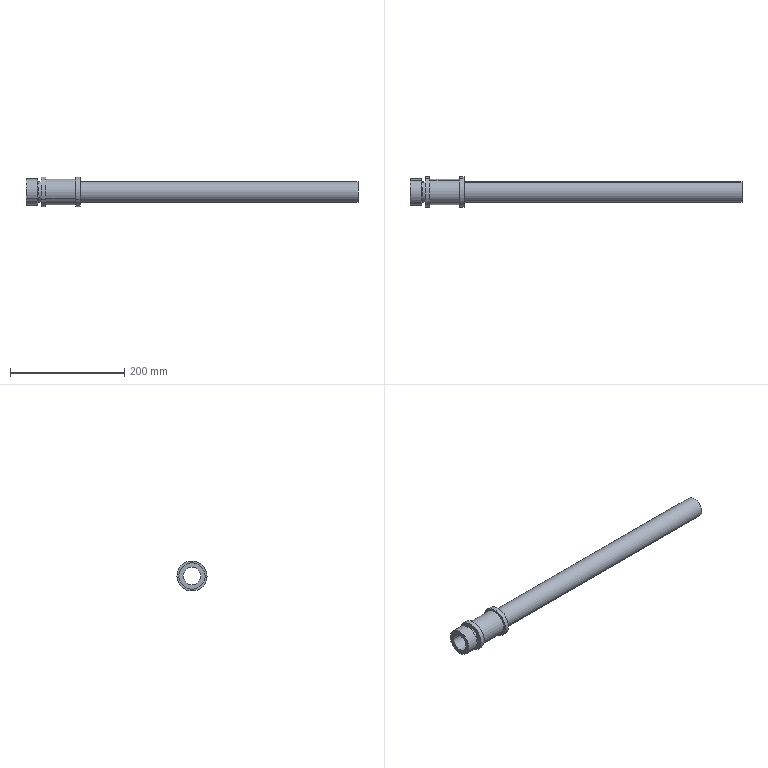Part | SolidWorks | features MBimport 1 | 1 solid | 29 faces | box 580 x 52.513 x 52.513 mm | volume 240293 mm3 | cylinder 20 | plane 6 | cone 3 | commonest cylinder face diameters 52.513 x6 36 x3 36.513 x3 44.513 x3 46 x3 30 x2
STEP:
#1=CARTESIAN_POINT('',(20.,23.,0.));
#2=VERTEX_POINT('',#1);
#3=CARTESIAN_POINT('',(20.,20.184,11.027));
#4=VERTEX_POINT('',#3);
#5=CARTESIAN_POINT('',(20.,0.,0.));
#6=DIRECTION('',(1.,0.,0.));
#7=DIRECTION('',(0.,1.,0.));
#8=AXIS2_PLACEMENT_3D('',#5,#6,#7);
#9=CIRCLE('',#8,23.);
#10=EDGE_CURVE('',#2,#4,#9,.T.);
#11=ORIENTED_EDGE('',*,*,#10,.F.);
#12=CARTESIAN_POINT('',(0.,23.,0.));
#13=VERTEX_POINT('',#12);
#14=CARTESIAN_POINT('',(190.,23.,0.));
#15=DIRECTION('',(-1.,0.,0.));
#16=VECTOR('',#15,1000.);
#17=LINE('',#14,#16);
#18=EDGE_CURVE('',#2,#13,#17,.T.);
#19=ORIENTED_EDGE('',*,*,#18,.T.);
#20=CARTESIAN_POINT('',(0.,20.184,11.027));
#21=VERTEX_POINT('',#20);
#22=CARTESIAN_POINT('',(0.,0.,0.));
#23=DIRECTION('',(1.,0.,0.));
#24=DIRECTION('',(0.,1.,0.));
#25=AXIS2_PLACEMENT_3D('',#22,#23,#24);
#26=CIRCLE('',#25,23.);
#27=EDGE_CURVE('',#13,#21,#26,.T.);
#28=ORIENTED_EDGE('',*,*,#27,.T.);
#29=CARTESIAN_POINT('',(10.,20.184,11.027));
#30=DIRECTION('',(-1.,0.,0.));
#31=VECTOR('',#30,1000.);
#32=LINE('',#29,#31);
#33=EDGE_CURVE('',#4,#21,#32,.T.);
#34=ORIENTED_EDGE('',*,*,#33,.F.);
#35=EDGE_LOOP('',(#11,#19,#28,#34));
#36=FACE_OUTER_BOUND('',#35,.T.);
#37=CARTESIAN_POINT('',(190.,0.,0.));
#38=DIRECTION('',(-1.,0.,0.));
#39=DIRECTION('',(0.,1.,0.));
#40=AXIS2_PLACEMENT_3D('',#37,#38,#39);
#41=CYLINDRICAL_SURFACE('',#40,23.);
#42=ADVANCED_FACE('',(#36),#41,.T.);
#43=CARTESIAN_POINT('',(21.582,18.257,0.));
#44=VERTEX_POINT('',#43);
#45=CARTESIAN_POINT('',(21.582,16.022,8.753));
#46=VERTEX_POINT('',#45);
#47=CARTESIAN_POINT('',(21.582,0.,0.));
#48=DIRECTION('',(1.,0.,0.));
#49=DIRECTION('',(0.,1.,0.));
#50=AXIS2_PLACEMENT_3D('',#47,#48,#49);
#51=CIRCLE('',#50,18.257);
#52=EDGE_CURVE('',#44,#46,#51,.T.);
#53=ORIENTED_EDGE('',*,*,#52,.F.);
#54=CARTESIAN_POINT('',(21.582,18.257,0.));
#55=DIRECTION('',(-0.3163,0.9487,0.));
#56=VECTOR('',#55,1000.);
#57=LINE('',#54,#56);
#58=EDGE_CURVE('',#44,#2,#57,.T.);
#59=ORIENTED_EDGE('',*,*,#58,.T.);
#60=ORIENTED_EDGE('',*,*,#10,.T.);
#61=CARTESIAN_POINT('',(20.791,18.103,9.89));
#62=DIRECTION('',(-0.3163,0.8325,0.4548));
#63=VECTOR('',#62,1000.);
#64=LINE('',#61,#63);
#65=EDGE_CURVE('',#46,#4,#64,.T.);
#66=ORIENTED_EDGE('',*,*,#65,.F.);
#67=EDGE_LOOP('',(#53,#59,#60,#66));
#68=FACE_OUTER_BOUND('',#67,.T.);
#69=CARTESIAN_POINT('',(21.582,0.,0.));
#70=DIRECTION('',(-1.,0.,0.));
#71=DIRECTION('',(0.,1.,0.));
#72=AXIS2_PLACEMENT_3D('',#69,#70,#71);
#73=CONICAL_SURFACE('',#72,18.257,1.249);
#74=ADVANCED_FACE('',(#68),#73,.T.);
#75=CARTESIAN_POINT('',(26.582,18.257,0.));
#76=VERTEX_POINT('',#75);
#77=CARTESIAN_POINT('',(26.582,16.022,8.753));
#78=VERTEX_POINT('',#77);
#79=CARTESIAN_POINT('',(26.582,0.,0.));
#80=DIRECTION('',(1.,0.,0.));
#81=DIRECTION('',(0.,1.,0.));
#82=AXIS2_PLACEMENT_3D('',#79,#80,#81);
#83=CIRCLE('',#82,18.257);
#84=EDGE_CURVE('',#76,#78,#83,.T.);
#85=ORIENTED_EDGE('',*,*,#84,.F.);
#86=CARTESIAN_POINT('',(190.,18.257,0.));
#87=DIRECTION('',(-1.,0.,0.));
#88=VECTOR('',#87,1000.);
#89=LINE('',#86,#88);
#90=EDGE_CURVE('',#76,#44,#89,.T.);
#91=ORIENTED_EDGE('',*,*,#90,.T.);
#92=ORIENTED_EDGE('',*,*,#52,.T.);
#93=CARTESIAN_POINT('',(24.082,16.022,8.753));
#94=DIRECTION('',(-1.,0.,0.));
#95=VECTOR('',#94,1000.);
#96=LINE('',#93,#95);
#97=EDGE_CURVE('',#78,#46,#96,.T.);
#98=ORIENTED_EDGE('',*,*,#97,.F.);
#99=EDGE_LOOP('',(#85,#91,#92,#98));
#100=FACE_OUTER_BOUND('',#99,.T.);
#101=CARTESIAN_POINT('',(190.,0.,0.));
#102=DIRECTION('',(-1.,0.,0.));
#103=DIRECTION('',(0.,1.,0.));
#104=AXIS2_PLACEMENT_3D('',#101,#102,#103);
#105=CYLINDRICAL_SURFACE('',#104,18.257);
#106=ADVANCED_FACE('',(#100),#105,.T.);
#107=CARTESIAN_POINT('',(34.582,26.257,0.));
#108=VERTEX_POINT('',#107);
#109=CARTESIAN_POINT('',(34.582,23.042,12.588));
#110=VERTEX_POINT('',#109);
#111=CARTESIAN_POINT('',(34.582,0.,0.));
#112=DIRECTION('',(1.,0.,0.));
#113=DIRECTION('',(0.,1.,0.));
#114=AXIS2_PLACEMENT_3D('',#111,#112,#113);
#115=CIRCLE('',#114,26.257);
#116=EDGE_CURVE('',#108,#110,#115,.T.);
#117=ORIENTED_EDGE('',*,*,#116,.F.);
#118=CARTESIAN_POINT('',(26.582,26.257,0.));
#119=VERTEX_POINT('',#118);
#120=CARTESIAN_POINT('',(190.,26.257,0.));
#121=DIRECTION('',(-1.,0.,0.));
#122=VECTOR('',#121,1000.);
#123=LINE('',#120,#122);
#124=EDGE_CURVE('',#108,#119,#123,.T.);
#125=ORIENTED_EDGE('',*,*,#124,.T.);
#126=CARTESIAN_POINT('',(26.582,23.042,12.588));
#127=VERTEX_POINT('',#126);
#128=CARTESIAN_POINT('',(26.582,0.,0.));
#129=DIRECTION('',(1.,0.,0.));
#130=DIRECTION('',(0.,1.,0.));
#131=AXIS2_PLACEMENT_3D('',#128,#129,#130);
#132=CIRCLE('',#131,26.257);
#133=EDGE_CURVE('',#119,#127,#132,.T.);
#134=ORIENTED_EDGE('',*,*,#133,.T.);
#135=CARTESIAN_POINT('',(60.582,23.042,12.588));
#136=DIRECTION('',(-1.,0.,0.));
#137=VECTOR('',#136,1000.);
#138=LINE('',#135,#137);
#139=EDGE_CURVE('',#110,#127,#138,.T.);
#140=ORIENTED_EDGE('',*,*,#139,.F.);
#141=EDGE_LOOP('',(#117,#125,#134,#140));
#142=FACE_OUTER_BOUND('',#141,.T.);
#143=CARTESIAN_POINT('',(190.,0.,0.));
#144=DIRECTION('',(-1.,0.,0.));
#145=DIRECTION('',(0.,1.,0.));
#146=AXIS2_PLACEMENT_3D('',#143,#144,#145);
#147=CYLINDRICAL_SURFACE('',#146,26.257);
#148=ADVANCED_FACE('',(#142),#147,.T.);
#149=CARTESIAN_POINT('',(86.582,22.257,0.));
#150=VERTEX_POINT('',#149);
#151=CARTESIAN_POINT('',(86.582,19.532,10.67));
#152=VERTEX_POINT('',#151);
#153=CARTESIAN_POINT('',(86.582,0.,0.));
#154=DIRECTION('',(1.,0.,0.));
#155=DIRECTION('',(0.,1.,0.));
#156=AXIS2_PLACEMENT_3D('',#153,#154,#155);
#157=CIRCLE('',#156,22.257);
#158=EDGE_CURVE('',#150,#152,#157,.T.);
#159=ORIENTED_EDGE('',*,*,#158,.F.);
#160=CARTESIAN_POINT('',(34.582,22.257,0.));
#161=VERTEX_POINT('',#160);
#162=CARTESIAN_POINT('',(190.,22.257,0.));
#163=DIRECTION('',(-1.,0.,0.));
#164=VECTOR('',#163,1000.);
#165=LINE('',#162,#164);
#166=EDGE_CURVE('',#150,#161,#165,.T.);
#167=ORIENTED_EDGE('',*,*,#166,.T.);
#168=CARTESIAN_POINT('',(34.582,19.532,10.67));
#169=VERTEX_POINT('',#168);
#170=CARTESIAN_POINT('',(34.582,0.,0.));
#171=DIRECTION('',(1.,0.,0.));
#172=DIRECTION('',(0.,1.,0.));
#173=AXIS2_PLACEMENT_3D('',#170,#171,#172);
#174=CIRCLE('',#173,22.257);
#175=EDGE_CURVE('',#161,#169,#174,.T.);
#176=ORIENTED_EDGE('',*,*,#175,.T.);
#177=CARTESIAN_POINT('',(60.582,19.532,10.67));
#178=DIRECTION('',(-1.,0.,0.));
#179=VECTOR('',#178,1000.);
#180=LINE('',#177,#179);
#181=EDGE_CURVE('',#152,#169,#180,.T.);
#182=ORIENTED_EDGE('',*,*,#181,.F.);
#183=EDGE_LOOP('',(#159,#167,#176,#182));
#184=FACE_OUTER_BOUND('',#183,.T.);
#185=CARTESIAN_POINT('',(190.,0.,0.));
#186=DIRECTION('',(-1.,0.,0.));
#187=DIRECTION('',(0.,1.,0.));
#188=AXIS2_PLACEMENT_3D('',#185,#186,#187);
#189=CYLINDRICAL_SURFACE('',#188,22.257);
#190=ADVANCED_FACE('',(#184),#189,.T.);
#191=CARTESIAN_POINT('',(94.582,26.257,0.));
#192=VERTEX_POINT('',#191);
#193=CARTESIAN_POINT('',(94.582,23.042,12.588));
#194=VERTEX_POINT('',#193);
#195=CARTESIAN_POINT('',(94.582,0.,0.));
#196=DIRECTION('',(1.,0.,0.));
#197=DIRECTION('',(0.,1.,0.));
#198=AXIS2_PLACEMENT_3D('',#195,#196,#197);
#199=CIRCLE('',#198,26.257);
#200=EDGE_CURVE('',#192,#194,#199,.T.);
#201=ORIENTED_EDGE('',*,*,#200,.F.);
#202=CARTESIAN_POINT('',(86.582,26.257,0.));
#203=VERTEX_POINT('',#202);
#204=CARTESIAN_POINT('',(190.,26.257,0.));
#205=DIRECTION('',(-1.,0.,0.));
#206=VECTOR('',#205,1000.);
#207=LINE('',#204,#206);
#208=EDGE_CURVE('',#192,#203,#207,.T.);
#209=ORIENTED_EDGE('',*,*,#208,.T.);
#210=CARTESIAN_POINT('',(86.582,23.042,12.588));
#211=VERTEX_POINT('',#210);
#212=CARTESIAN_POINT('',(86.582,0.,0.));
#213=DIRECTION('',(1.,0.,0.));
#214=DIRECTION('',(0.,1.,0.));
#215=AXIS2_PLACEMENT_3D('',#212,#213,#214);
#216=CIRCLE('',#215,26.257);
#217=EDGE_CURVE('',#203,#211,#216,.T.);
#218=ORIENTED_EDGE('',*,*,#217,.T.);
#219=CARTESIAN_POINT('',(60.582,23.042,12.588));
#220=DIRECTION('',(-1.,0.,0.));
#221=VECTOR('',#220,1000.);
#222=LINE('',#219,#221);
#223=EDGE_CURVE('',#194,#211,#222,.T.);
#224=ORIENTED_EDGE('',*,*,#223,.F.);
#225=EDGE_LOOP('',(#201,#209,#218,#224));
#226=FACE_OUTER_BOUND('',#225,.T.);
#227=CARTESIAN_POINT('',(190.,0.,0.));
#228=DIRECTION('',(-1.,0.,0.));
#229=DIRECTION('',(0.,1.,0.));
#230=AXIS2_PLACEMENT_3D('',#227,#228,#229);
#231=CYLINDRICAL_SURFACE('',#230,26.257);
#232=ADVANCED_FACE('',(#226),#231,.T.);
#233=CARTESIAN_POINT('',(580.,18.,0.));
#234=VERTEX_POINT('',#233);
#235=CARTESIAN_POINT('',(580.,15.796,8.63));
#236=VERTEX_POINT('',#235);
#237=CARTESIAN_POINT('',(580.,0.,0.));
#238=DIRECTION('',(1.,0.,0.));
#239=DIRECTION('',(0.,1.,0.));
#240=AXIS2_PLACEMENT_3D('',#237,#238,#239);
#241=CIRCLE('',#240,18.);
#242=EDGE_CURVE('',#234,#236,#241,.T.);
#243=ORIENTED_EDGE('',*,*,#242,.F.);
#244=CARTESIAN_POINT('',(94.582,18.,0.));
#245=VERTEX_POINT('',#244);
#246=CARTESIAN_POINT('',(190.,18.,0.));
#247=DIRECTION('',(-1.,0.,0.));
#248=VECTOR('',#247,1000.);
#249=LINE('',#246,#248);
#250=EDGE_CURVE('',#234,#245,#249,.T.);
#251=ORIENTED_EDGE('',*,*,#250,.T.);
#252=CARTESIAN_POINT('',(94.582,15.796,8.63));
#253=VERTEX_POINT('',#252);
#254=CARTESIAN_POINT('',(94.582,0.,0.));
#255=DIRECTION('',(1.,0.,0.));
#256=DIRECTION('',(0.,1.,0.));
#257=AXIS2_PLACEMENT_3D('',#254,#255,#256);
#258=CIRCLE('',#257,18.);
#259=EDGE_CURVE('',#245,#253,#258,.T.);
#260=ORIENTED_EDGE('',*,*,#259,.T.);
#261=CARTESIAN_POINT('',(337.291,15.796,8.63));
#262=DIRECTION('',(-1.,0.,0.));
#263=VECTOR('',#262,1000.);
#264=LINE('',#261,#263);
#265=EDGE_CURVE('',#236,#253,#264,.T.);
#266=ORIENTED_EDGE('',*,*,#265,.F.);
#267=EDGE_LOOP('',(#243,#251,#260,#266));
#268=FACE_OUTER_BOUND('',#267,.T.);
#269=CARTESIAN_POINT('',(190.,0.,0.));
#270=DIRECTION('',(-1.,0.,0.));
#271=DIRECTION('',(0.,1.,0.));
#272=AXIS2_PLACEMENT_3D('',#269,#270,#271);
#273=CYLINDRICAL_SURFACE('',#272,18.);
#274=ADVANCED_FACE('',(#268),#273,.T.);
#275=CARTESIAN_POINT('',(94.582,-15.796,-8.63));
#276=VERTEX_POINT('',#275);
#277=CARTESIAN_POINT('',(94.582,0.,0.));
#278=DIRECTION('',(1.,0.,0.));
#279=DIRECTION('',(0.,1.,0.));
#280=AXIS2_PLACEMENT_3D('',#277,#278,#279);
#281=CIRCLE('',#280,18.);
#282=EDGE_CURVE('',#253,#276,#281,.T.);
#283=ORIENTED_EDGE('',*,*,#282,.F.);
#284=ORIENTED_EDGE('',*,*,#259,.F.);
#285=CARTESIAN_POINT('',(94.582,0.,0.));
#286=DIRECTION('',(1.,0.,0.));
#287=DIRECTION('',(0.,1.,0.));
#288=AXIS2_PLACEMENT_3D('',#285,#286,#287);
#289=CIRCLE('',#288,18.);
#290=EDGE_CURVE('',#276,#245,#289,.T.);
#291=ORIENTED_EDGE('',*,*,#290,.F.);
#292=EDGE_LOOP('',(#283,#284,#291));
#293=FACE_BOUND('',#292,.T.);
#294=CARTESIAN_POINT('',(94.582,-23.042,-12.588));
#295=VERTEX_POINT('',#294);
#296=CARTESIAN_POINT('',(94.582,0.,0.));
#297=DIRECTION('',(1.,0.,0.));
#298=DIRECTION('',(0.,1.,0.));
#299=AXIS2_PLACEMENT_3D('',#296,#297,#298);
#300=CIRCLE('',#299,26.257);
#301=EDGE_CURVE('',#295,#192,#300,.T.);
#302=ORIENTED_EDGE('',*,*,#301,.T.);
#303=ORIENTED_EDGE('',*,*,#200,.T.);
#304=CARTESIAN_POINT('',(94.582,0.,0.));
#305=DIRECTION('',(1.,0.,0.));
#306=DIRECTION('',(0.,1.,0.));
#307=AXIS2_PLACEMENT_3D('',#304,#305,#306);
#308=CIRCLE('',#307,26.257);
#309=EDGE_CURVE('',#194,#295,#308,.T.);
#310=ORIENTED_EDGE('',*,*,#309,.T.);
#311=EDGE_LOOP('',(#302,#303,#310));
#312=FACE_OUTER_BOUND('',#311,.T.);
#313=CARTESIAN_POINT('',(94.582,26.257,0.));
#314=DIRECTION('',(1.,0.,0.));
#315=DIRECTION('',(0.,1.,0.));
#316=AXIS2_PLACEMENT_3D('',#313,#314,#315);
#317=PLANE('',#316);
#318=ADVANCED_FACE('',(#293,#312),#317,.T.);
#319=CARTESIAN_POINT('',(580.,15.,0.));
#320=VERTEX_POINT('',#319);
#321=CARTESIAN_POINT('',(580.,-15.,0.));
#322=VERTEX_POINT('',#321);
#323=CARTESIAN_POINT('',(580.,0.,0.));
#324=DIRECTION('',(1.,0.,0.));
#325=DIRECTION('',(0.,1.,0.));
#326=AXIS2_PLACEMENT_3D('',#323,#324,#325);
#327=CIRCLE('',#326,15.);
#328=EDGE_CURVE('',#320,#322,#327,.T.);
#329=ORIENTED_EDGE('',*,*,#328,.F.);
#330=CARTESIAN_POINT('',(580.,0.,0.));
#331=DIRECTION('',(1.,0.,0.));
#332=DIRECTION('',(0.,1.,0.));
#333=AXIS2_PLACEMENT_3D('',#330,#331,#332);
#334=CIRCLE('',#333,15.);
#335=EDGE_CURVE('',#322,#320,#334,.T.);
#336=ORIENTED_EDGE('',*,*,#335,.F.);
#337=EDGE_LOOP('',(#329,#336));
#338=FACE_BOUND('',#337,.T.);
#339=CARTESIAN_POINT('',(580.,-15.796,-8.63));
#340=VERTEX_POINT('',#339);
#341=CARTESIAN_POINT('',(580.,0.,0.));
#342=DIRECTION('',(1.,0.,0.));
#343=DIRECTION('',(0.,1.,0.));
#344=AXIS2_PLACEMENT_3D('',#341,#342,#343);
#345=CIRCLE('',#344,18.);
#346=EDGE_CURVE('',#236,#340,#345,.T.);
#347=ORIENTED_EDGE('',*,*,#346,.T.);
#348=CARTESIAN_POINT('',(580.,0.,0.));
#349=DIRECTION('',(1.,0.,0.));
#350=DIRECTION('',(0.,1.,0.));
#351=AXIS2_PLACEMENT_3D('',#348,#349,#350);
#352=CIRCLE('',#351,18.);
#353=EDGE_CURVE('',#340,#234,#352,.T.);
#354=ORIENTED_EDGE('',*,*,#353,.T.);
#355=ORIENTED_EDGE('',*,*,#242,.T.);
#356=EDGE_LOOP('',(#347,#354,#355));
#357=FACE_OUTER_BOUND('',#356,.T.);
#358=CARTESIAN_POINT('',(580.,0.,0.));
#359=DIRECTION('',(1.,0.,0.));
#360=DIRECTION('',(0.,1.,0.));
#361=AXIS2_PLACEMENT_3D('',#358,#359,#360);
#362=PLANE('',#361);
#363=ADVANCED_FACE('',(#338,#357),#362,.T.);
#364=ORIENTED_EDGE('',*,*,#265,.T.);
#365=ORIENTED_EDGE('',*,*,#282,.T.);
#366=CARTESIAN_POINT('',(337.291,-15.796,-8.63));
#367=DIRECTION('',(-1.,0.,0.));
#368=VECTOR('',#367,1000.);
#369=LINE('',#366,#368);
#370=EDGE_CURVE('',#340,#276,#369,.T.);
#371=ORIENTED_EDGE('',*,*,#370,.F.);
#372=ORIENTED_EDGE('',*,*,#346,.F.);
#373=EDGE_LOOP('',(#364,#365,#371,#372));
#374=FACE_OUTER_BOUND('',#373,.T.);
#375=CARTESIAN_POINT('',(190.,0.,0.));
#376=DIRECTION('',(-1.,0.,0.));
#377=DIRECTION('',(0.,1.,0.));
#378=AXIS2_PLACEMENT_3D('',#375,#376,#377);
#379=CYLINDRICAL_SURFACE('',#378,18.);
#380=ADVANCED_FACE('',(#374),#379,.T.);
#381=ORIENTED_EDGE('',*,*,#250,.F.);
#382=ORIENTED_EDGE('',*,*,#353,.F.);
#383=ORIENTED_EDGE('',*,*,#370,.T.);
#384=ORIENTED_EDGE('',*,*,#290,.T.);
#385=EDGE_LOOP('',(#381,#382,#383,#384));
#386=FACE_OUTER_BOUND('',#385,.T.);
#387=CARTESIAN_POINT('',(190.,0.,0.));
#388=DIRECTION('',(-1.,0.,0.));
#389=DIRECTION('',(0.,1.,0.));
#390=AXIS2_PLACEMENT_3D('',#387,#388,#389);
#391=CYLINDRICAL_SURFACE('',#390,18.);
#392=ADVANCED_FACE('',(#386),#391,.T.);
#393=ORIENTED_EDGE('',*,*,#335,.T.);
#394=CARTESIAN_POINT('',(0.,15.,0.));
#395=VERTEX_POINT('',#394);
#396=CARTESIAN_POINT('',(530.,15.,0.));
#397=DIRECTION('',(-1.,0.,0.));
#398=VECTOR('',#397,1000.);
#399=LINE('',#396,#398);
#400=EDGE_CURVE('',#320,#395,#399,.T.);
#401=ORIENTED_EDGE('',*,*,#400,.T.);
#402=CARTESIAN_POINT('',(0.,-15.,0.));
#403=VERTEX_POINT('',#402);
#404=CARTESIAN_POINT('',(0.,0.,0.));
#405=DIRECTION('',(1.,0.,0.));
#406=DIRECTION('',(0.,1.,0.));
#407=AXIS2_PLACEMENT_3D('',#404,#405,#406);
#408=CIRCLE('',#407,15.);
#409=EDGE_CURVE('',#403,#395,#408,.T.);
#410=ORIENTED_EDGE('',*,*,#409,.F.);
#411=CARTESIAN_POINT('',(530.,-15.,0.));
#412=DIRECTION('',(-1.,0.,0.));
#413=VECTOR('',#412,1000.);
#414=LINE('',#411,#413);
#415=EDGE_CURVE('',#322,#403,#414,.T.);
#416=ORIENTED_EDGE('',*,*,#415,.F.);
#417=EDGE_LOOP('',(#393,#401,#410,#416));
#418=FACE_OUTER_BOUND('',#417,.T.);
#419=CARTESIAN_POINT('',(530.,0.,0.));
#420=DIRECTION('',(-1.,0.,0.));
#421=DIRECTION('',(0.,1.,0.));
#422=AXIS2_PLACEMENT_3D('',#419,#420,#421);
#423=CYLINDRICAL_SURFACE('',#422,15.);
#424=ADVANCED_FACE('',(#418),#423,.F.);
#425=ORIENTED_EDGE('',*,*,#328,.T.);
#426=ORIENTED_EDGE('',*,*,#415,.T.);
#427=CARTESIAN_POINT('',(0.,0.,0.));
#428=DIRECTION('',(1.,0.,0.));
#429=DIRECTION('',(0.,1.,0.));
#430=AXIS2_PLACEMENT_3D('',#427,#428,#429);
#431=CIRCLE('',#430,15.);
#432=EDGE_CURVE('',#395,#403,#431,.T.);
#433=ORIENTED_EDGE('',*,*,#432,.F.);
#434=ORIENTED_EDGE('',*,*,#400,.F.);
#435=EDGE_LOOP('',(#425,#426,#433,#434));
#436=FACE_OUTER_BOUND('',#435,.T.);
#437=CARTESIAN_POINT('',(530.,0.,0.));
#438=DIRECTION('',(-1.,0.,0.));
#439=DIRECTION('',(0.,1.,0.));
#440=AXIS2_PLACEMENT_3D('',#437,#438,#439);
#441=CYLINDRICAL_SURFACE('',#440,15.);
#442=ADVANCED_FACE('',(#436),#441,.F.);
#443=ORIENTED_EDGE('',*,*,#409,.T.);
#444=ORIENTED_EDGE('',*,*,#432,.T.);
#445=EDGE_LOOP('',(#443,#444));
#446=FACE_BOUND('',#445,.T.);
#447=CARTESIAN_POINT('',(0.,-20.184,-11.027));
#448=VERTEX_POINT('',#447);
#449=CARTESIAN_POINT('',(0.,0.,0.));
#450=DIRECTION('',(1.,0.,0.));
#451=DIRECTION('',(0.,1.,0.));
#452=AXIS2_PLACEMENT_3D('',#449,#450,#451);
#453=CIRCLE('',#452,23.);
#454=EDGE_CURVE('',#21,#448,#453,.T.);
#455=ORIENTED_EDGE('',*,*,#454,.F.);
#456=ORIENTED_EDGE('',*,*,#27,.F.);
#457=CARTESIAN_POINT('',(0.,0.,0.));
#458=DIRECTION('',(1.,0.,0.));
#459=DIRECTION('',(0.,1.,0.));
#460=AXIS2_PLACEMENT_3D('',#457,#458,#459);
#461=CIRCLE('',#460,23.);
#462=EDGE_CURVE('',#448,#13,#461,.T.);
#463=ORIENTED_EDGE('',*,*,#462,.F.);
#464=EDGE_LOOP('',(#455,#456,#463));
#465=FACE_OUTER_BOUND('',#464,.T.);
#466=CARTESIAN_POINT('',(0.,0.,0.));
#467=DIRECTION('',(1.,0.,0.));
#468=DIRECTION('',(0.,1.,0.));
#469=AXIS2_PLACEMENT_3D('',#466,#467,#468);
#470=PLANE('',#469);
#471=ADVANCED_FACE('',(#446,#465),#470,.F.);
#472=ORIENTED_EDGE('',*,*,#309,.F.);
#473=ORIENTED_EDGE('',*,*,#223,.T.);
#474=CARTESIAN_POINT('',(86.582,-23.042,-12.588));
#475=VERTEX_POINT('',#474);
#476=CARTESIAN_POINT('',(86.582,0.,0.));
#477=DIRECTION('',(1.,0.,0.));
#478=DIRECTION('',(0.,1.,0.));
#479=AXIS2_PLACEMENT_3D('',#476,#477,#478);
#480=CIRCLE('',#479,26.257);
#481=EDGE_CURVE('',#211,#475,#480,.T.);
#482=ORIENTED_EDGE('',*,*,#481,.T.);
#483=CARTESIAN_POINT('',(60.582,-23.042,-12.588));
#484=DIRECTION('',(-1.,0.,0.));
#485=VECTOR('',#484,1000.);
#486=LINE('',#483,#485);
#487=EDGE_CURVE('',#295,#475,#486,.T.);
#488=ORIENTED_EDGE('',*,*,#487,.F.);
#489=EDGE_LOOP('',(#472,#473,#482,#488));
#490=FACE_OUTER_BOUND('',#489,.T.);
#491=CARTESIAN_POINT('',(190.,0.,0.));
#492=DIRECTION('',(-1.,0.,0.));
#493=DIRECTION('',(0.,1.,0.));
#494=AXIS2_PLACEMENT_3D('',#491,#492,#493);
#495=CYLINDRICAL_SURFACE('',#494,26.257);
#496=ADVANCED_FACE('',(#490),#495,.T.);
#497=ORIENTED_EDGE('',*,*,#208,.F.);
#498=ORIENTED_EDGE('',*,*,#301,.F.);
#499=ORIENTED_EDGE('',*,*,#487,.T.);
#500=CARTESIAN_POINT('',(86.582,0.,0.));
#501=DIRECTION('',(1.,0.,0.));
#502=DIRECTION('',(0.,1.,0.));
#503=AXIS2_PLACEMENT_3D('',#500,#501,#502);
#504=CIRCLE('',#503,26.257);
#505=EDGE_CURVE('',#475,#203,#504,.T.);
#506=ORIENTED_EDGE('',*,*,#505,.T.);
#507=EDGE_LOOP('',(#497,#498,#499,#506));
#508=FACE_OUTER_BOUND('',#507,.T.);
#509=CARTESIAN_POINT('',(190.,0.,0.));
#510=DIRECTION('',(-1.,0.,0.));
#511=DIRECTION('',(0.,1.,0.));
#512=AXIS2_PLACEMENT_3D('',#509,#510,#511);
#513=CYLINDRICAL_SURFACE('',#512,26.257);
#514=ADVANCED_FACE('',(#508),#513,.T.);
#515=CARTESIAN_POINT('',(86.582,-19.532,-10.67));
#516=VERTEX_POINT('',#515);
#517=CARTESIAN_POINT('',(86.582,0.,0.));
#518=DIRECTION('',(1.,0.,0.));
#519=DIRECTION('',(0.,1.,0.));
#520=AXIS2_PLACEMENT_3D('',#517,#518,#519);
#521=CIRCLE('',#520,22.257);
#522=EDGE_CURVE('',#516,#150,#521,.T.);
#523=ORIENTED_EDGE('',*,*,#522,.T.);
#524=ORIENTED_EDGE('',*,*,#158,.T.);
#525=CARTESIAN_POINT('',(86.582,0.,0.));
#526=DIRECTION('',(1.,0.,0.));
#527=DIRECTION('',(0.,1.,0.));
#528=AXIS2_PLACEMENT_3D('',#525,#526,#527);
#529=CIRCLE('',#528,22.257);
#530=EDGE_CURVE('',#152,#516,#529,.T.);
#531=ORIENTED_EDGE('',*,*,#530,.T.);
#532=EDGE_LOOP('',(#523,#524,#531));
#533=FACE_BOUND('',#532,.T.);
#534=ORIENTED_EDGE('',*,*,#481,.F.);
#535=ORIENTED_EDGE('',*,*,#217,.F.);
#536=ORIENTED_EDGE('',*,*,#505,.F.);
#537=EDGE_LOOP('',(#534,#535,#536));
#538=FACE_OUTER_BOUND('',#537,.T.);
#539=CARTESIAN_POINT('',(86.582,22.257,0.));
#540=DIRECTION('',(1.,0.,0.));
#541=DIRECTION('',(0.,1.,0.));
#542=AXIS2_PLACEMENT_3D('',#539,#540,#541);
#543=PLANE('',#542);
#544=ADVANCED_FACE('',(#533,#538),#543,.F.);
#545=ORIENTED_EDGE('',*,*,#166,.F.);
#546=ORIENTED_EDGE('',*,*,#522,.F.);
#547=CARTESIAN_POINT('',(34.582,-19.532,-10.67));
#548=VERTEX_POINT('',#547);
#549=CARTESIAN_POINT('',(60.582,-19.532,-10.67));
#550=DIRECTION('',(-1.,0.,0.));
#551=VECTOR('',#550,1000.);
#552=LINE('',#549,#551);
#553=EDGE_CURVE('',#516,#548,#552,.T.);
#554=ORIENTED_EDGE('',*,*,#553,.T.);
#555=CARTESIAN_POINT('',(34.582,0.,0.));
#556=DIRECTION('',(1.,0.,0.));
#557=DIRECTION('',(0.,1.,0.));
#558=AXIS2_PLACEMENT_3D('',#555,#556,#557);
#559=CIRCLE('',#558,22.257);
#560=EDGE_CURVE('',#548,#161,#559,.T.);
#561=ORIENTED_EDGE('',*,*,#560,.T.);
#562=EDGE_LOOP('',(#545,#546,#554,#561));
#563=FACE_OUTER_BOUND('',#562,.T.);
#564=CARTESIAN_POINT('',(190.,0.,0.));
#565=DIRECTION('',(-1.,0.,0.));
#566=DIRECTION('',(0.,1.,0.));
#567=AXIS2_PLACEMENT_3D('',#564,#565,#566);
#568=CYLINDRICAL_SURFACE('',#567,22.257);
#569=ADVANCED_FACE('',(#563),#568,.T.);
#570=ORIENTED_EDGE('',*,*,#530,.F.);
#571=ORIENTED_EDGE('',*,*,#181,.T.);
#572=CARTESIAN_POINT('',(34.582,0.,0.));
#573=DIRECTION('',(1.,0.,0.));
#574=DIRECTION('',(0.,1.,0.));
#575=AXIS2_PLACEMENT_3D('',#572,#573,#574);
#576=CIRCLE('',#575,22.257);
#577=EDGE_CURVE('',#169,#548,#576,.T.);
#578=ORIENTED_EDGE('',*,*,#577,.T.);
#579=ORIENTED_EDGE('',*,*,#553,.F.);
#580=EDGE_LOOP('',(#570,#571,#578,#579));
#581=FACE_OUTER_BOUND('',#580,.T.);
#582=CARTESIAN_POINT('',(190.,0.,0.));
#583=DIRECTION('',(-1.,0.,0.));
#584=DIRECTION('',(0.,1.,0.));
#585=AXIS2_PLACEMENT_3D('',#582,#583,#584);
#586=CYLINDRICAL_SURFACE('',#585,22.257);
#587=ADVANCED_FACE('',(#581),#586,.T.);
#588=ORIENTED_EDGE('',*,*,#577,.F.);
#589=ORIENTED_EDGE('',*,*,#175,.F.);
#590=ORIENTED_EDGE('',*,*,#560,.F.);
#591=EDGE_LOOP('',(#588,#589,#590));
#592=FACE_BOUND('',#591,.T.);
#593=CARTESIAN_POINT('',(34.582,-23.042,-12.588));
#594=VERTEX_POINT('',#593);
#595=CARTESIAN_POINT('',(34.582,0.,0.));
#596=DIRECTION('',(1.,0.,0.));
#597=DIRECTION('',(0.,1.,0.));
#598=AXIS2_PLACEMENT_3D('',#595,#596,#597);
#599=CIRCLE('',#598,26.257);
#600=EDGE_CURVE('',#594,#108,#599,.T.);
#601=ORIENTED_EDGE('',*,*,#600,.T.);
#602=ORIENTED_EDGE('',*,*,#116,.T.);
#603=CARTESIAN_POINT('',(34.582,0.,0.));
#604=DIRECTION('',(1.,0.,0.));
#605=DIRECTION('',(0.,1.,0.));
#606=AXIS2_PLACEMENT_3D('',#603,#604,#605);
#607=CIRCLE('',#606,26.257);
#608=EDGE_CURVE('',#110,#594,#607,.T.);
#609=ORIENTED_EDGE('',*,*,#608,.T.);
#610=EDGE_LOOP('',(#601,#602,#609));
#611=FACE_OUTER_BOUND('',#610,.T.);
#612=CARTESIAN_POINT('',(34.582,26.257,0.));
#613=DIRECTION('',(1.,0.,0.));
#614=DIRECTION('',(0.,1.,0.));
#615=AXIS2_PLACEMENT_3D('',#612,#613,#614);
#616=PLANE('',#615);
#617=ADVANCED_FACE('',(#592,#611),#616,.T.);
#618=ORIENTED_EDGE('',*,*,#608,.F.);
#619=ORIENTED_EDGE('',*,*,#139,.T.);
#620=CARTESIAN_POINT('',(26.582,-23.042,-12.588));
#621=VERTEX_POINT('',#620);
#622=CARTESIAN_POINT('',(26.582,0.,0.));
#623=DIRECTION('',(1.,0.,0.));
#624=DIRECTION('',(0.,1.,0.));
#625=AXIS2_PLACEMENT_3D('',#622,#623,#624);
#626=CIRCLE('',#625,26.257);
#627=EDGE_CURVE('',#127,#621,#626,.T.);
#628=ORIENTED_EDGE('',*,*,#627,.T.);
#629=CARTESIAN_POINT('',(60.582,-23.042,-12.588));
#630=DIRECTION('',(-1.,0.,0.));
#631=VECTOR('',#630,1000.);
#632=LINE('',#629,#631);
#633=EDGE_CURVE('',#594,#621,#632,.T.);
#634=ORIENTED_EDGE('',*,*,#633,.F.);
#635=EDGE_LOOP('',(#618,#619,#628,#634));
#636=FACE_OUTER_BOUND('',#635,.T.);
#637=CARTESIAN_POINT('',(190.,0.,0.));
#638=DIRECTION('',(-1.,0.,0.));
#639=DIRECTION('',(0.,1.,0.));
#640=AXIS2_PLACEMENT_3D('',#637,#638,#639);
#641=CYLINDRICAL_SURFACE('',#640,26.257);
#642=ADVANCED_FACE('',(#636),#641,.T.);
#643=ORIENTED_EDGE('',*,*,#124,.F.);
#644=ORIENTED_EDGE('',*,*,#600,.F.);
#645=ORIENTED_EDGE('',*,*,#633,.T.);
#646=CARTESIAN_POINT('',(26.582,0.,0.));
#647=DIRECTION('',(1.,0.,0.));
#648=DIRECTION('',(0.,1.,0.));
#649=AXIS2_PLACEMENT_3D('',#646,#647,#648);
#650=CIRCLE('',#649,26.257);
#651=EDGE_CURVE('',#621,#119,#650,.T.);
#652=ORIENTED_EDGE('',*,*,#651,.T.);
#653=EDGE_LOOP('',(#643,#644,#645,#652));
#654=FACE_OUTER_BOUND('',#653,.T.);
#655=CARTESIAN_POINT('',(190.,0.,0.));
#656=DIRECTION('',(-1.,0.,0.));
#657=DIRECTION('',(0.,1.,0.));
#658=AXIS2_PLACEMENT_3D('',#655,#656,#657);
#659=CYLINDRICAL_SURFACE('',#658,26.257);
#660=ADVANCED_FACE('',(#654),#659,.T.);
#661=CARTESIAN_POINT('',(26.582,-16.022,-8.753));
#662=VERTEX_POINT('',#661);
#663=CARTESIAN_POINT('',(26.582,0.,0.));
#664=DIRECTION('',(1.,0.,0.));
#665=DIRECTION('',(0.,1.,0.));
#666=AXIS2_PLACEMENT_3D('',#663,#664,#665);
#667=CIRCLE('',#666,18.257);
#668=EDGE_CURVE('',#662,#76,#667,.T.);
#669=ORIENTED_EDGE('',*,*,#668,.T.);
#670=ORIENTED_EDGE('',*,*,#84,.T.);
#671=CARTESIAN_POINT('',(26.582,0.,0.));
#672=DIRECTION('',(1.,0.,0.));
#673=DIRECTION('',(0.,1.,0.));
#674=AXIS2_PLACEMENT_3D('',#671,#672,#673);
#675=CIRCLE('',#674,18.257);
#676=EDGE_CURVE('',#78,#662,#675,.T.);
#677=ORIENTED_EDGE('',*,*,#676,.T.);
#678=EDGE_LOOP('',(#669,#670,#677));
#679=FACE_BOUND('',#678,.T.);
#680=ORIENTED_EDGE('',*,*,#627,.F.);
#681=ORIENTED_EDGE('',*,*,#133,.F.);
#682=ORIENTED_EDGE('',*,*,#651,.F.);
#683=EDGE_LOOP('',(#680,#681,#682));
#684=FACE_OUTER_BOUND('',#683,.T.);
#685=CARTESIAN_POINT('',(26.582,18.257,0.));
#686=DIRECTION('',(1.,0.,0.));
#687=DIRECTION('',(0.,1.,0.));
#688=AXIS2_PLACEMENT_3D('',#685,#686,#687);
#689=PLANE('',#688);
#690=ADVANCED_FACE('',(#679,#684),#689,.F.);
#691=ORIENTED_EDGE('',*,*,#676,.F.);
#692=ORIENTED_EDGE('',*,*,#97,.T.);
#693=CARTESIAN_POINT('',(21.582,-16.022,-8.753));
#694=VERTEX_POINT('',#693);
#695=CARTESIAN_POINT('',(21.582,0.,0.));
#696=DIRECTION('',(1.,0.,0.));
#697=DIRECTION('',(0.,1.,0.));
#698=AXIS2_PLACEMENT_3D('',#695,#696,#697);
#699=CIRCLE('',#698,18.257);
#700=EDGE_CURVE('',#46,#694,#699,.T.);
#701=ORIENTED_EDGE('',*,*,#700,.T.);
#702=CARTESIAN_POINT('',(24.082,-16.022,-8.753));
#703=DIRECTION('',(-1.,0.,0.));
#704=VECTOR('',#703,1000.);
#705=LINE('',#702,#704);
#706=EDGE_CURVE('',#662,#694,#705,.T.);
#707=ORIENTED_EDGE('',*,*,#706,.F.);
#708=EDGE_LOOP('',(#691,#692,#701,#707));
#709=FACE_OUTER_BOUND('',#708,.T.);
#710=CARTESIAN_POINT('',(190.,0.,0.));
#711=DIRECTION('',(-1.,0.,0.));
#712=DIRECTION('',(0.,1.,0.));
#713=AXIS2_PLACEMENT_3D('',#710,#711,#712);
#714=CYLINDRICAL_SURFACE('',#713,18.257);
#715=ADVANCED_FACE('',(#709),#714,.T.);
#716=ORIENTED_EDGE('',*,*,#90,.F.);
#717=ORIENTED_EDGE('',*,*,#668,.F.);
#718=ORIENTED_EDGE('',*,*,#706,.T.);
#719=CARTESIAN_POINT('',(21.582,0.,0.));
#720=DIRECTION('',(1.,0.,0.));
#721=DIRECTION('',(0.,1.,0.));
#722=AXIS2_PLACEMENT_3D('',#719,#720,#721);
#723=CIRCLE('',#722,18.257);
#724=EDGE_CURVE('',#694,#44,#723,.T.);
#725=ORIENTED_EDGE('',*,*,#724,.T.);
#726=EDGE_LOOP('',(#716,#717,#718,#725));
#727=FACE_OUTER_BOUND('',#726,.T.);
#728=CARTESIAN_POINT('',(190.,0.,0.));
#729=DIRECTION('',(-1.,0.,0.));
#730=DIRECTION('',(0.,1.,0.));
#731=AXIS2_PLACEMENT_3D('',#728,#729,#730);
#732=CYLINDRICAL_SURFACE('',#731,18.257);
#733=ADVANCED_FACE('',(#727),#732,.T.);
#734=ORIENTED_EDGE('',*,*,#700,.F.);
#735=ORIENTED_EDGE('',*,*,#65,.T.);
#736=CARTESIAN_POINT('',(20.,-20.184,-11.027));
#737=VERTEX_POINT('',#736);
#738=CARTESIAN_POINT('',(20.,0.,0.));
#739=DIRECTION('',(1.,0.,0.));
#740=DIRECTION('',(0.,1.,0.));
#741=AXIS2_PLACEMENT_3D('',#738,#739,#740);
#742=CIRCLE('',#741,23.);
#743=EDGE_CURVE('',#4,#737,#742,.T.);
#744=ORIENTED_EDGE('',*,*,#743,.T.);
#745=CARTESIAN_POINT('',(20.791,-18.103,-9.89));
#746=DIRECTION('',(-0.3163,-0.8325,-0.4548));
#747=VECTOR('',#746,1000.);
#748=LINE('',#745,#747);
#749=EDGE_CURVE('',#694,#737,#748,.T.);
#750=ORIENTED_EDGE('',*,*,#749,.F.);
#751=EDGE_LOOP('',(#734,#735,#744,#750));
#752=FACE_OUTER_BOUND('',#751,.T.);
#753=CARTESIAN_POINT('',(21.582,0.,0.));
#754=DIRECTION('',(-1.,0.,0.));
#755=DIRECTION('',(0.,1.,0.));
#756=AXIS2_PLACEMENT_3D('',#753,#754,#755);
#757=CONICAL_SURFACE('',#756,18.257,1.249);
#758=ADVANCED_FACE('',(#752),#757,.T.);
#759=ORIENTED_EDGE('',*,*,#58,.F.);
#760=ORIENTED_EDGE('',*,*,#724,.F.);
#761=ORIENTED_EDGE('',*,*,#749,.T.);
#762=CARTESIAN_POINT('',(20.,0.,0.));
#763=DIRECTION('',(1.,0.,0.));
#764=DIRECTION('',(0.,1.,0.));
#765=AXIS2_PLACEMENT_3D('',#762,#763,#764);
#766=CIRCLE('',#765,23.);
#767=EDGE_CURVE('',#737,#2,#766,.T.);
#768=ORIENTED_EDGE('',*,*,#767,.T.);
#769=EDGE_LOOP('',(#759,#760,#761,#768));
#770=FACE_OUTER_BOUND('',#769,.T.);
#771=CARTESIAN_POINT('',(21.582,0.,0.));
#772=DIRECTION('',(-1.,0.,0.));
#773=DIRECTION('',(0.,1.,0.));
#774=AXIS2_PLACEMENT_3D('',#771,#772,#773);
#775=CONICAL_SURFACE('',#774,18.257,1.249);
#776=ADVANCED_FACE('',(#770),#775,.T.);
#777=ORIENTED_EDGE('',*,*,#743,.F.);
#778=ORIENTED_EDGE('',*,*,#33,.T.);
#779=ORIENTED_EDGE('',*,*,#454,.T.);
#780=CARTESIAN_POINT('',(10.,-20.184,-11.027));
#781=DIRECTION('',(-1.,0.,0.));
#782=VECTOR('',#781,1000.);
#783=LINE('',#780,#782);
#784=EDGE_CURVE('',#737,#448,#783,.T.);
#785=ORIENTED_EDGE('',*,*,#784,.F.);
#786=EDGE_LOOP('',(#777,#778,#779,#785));
#787=FACE_OUTER_BOUND('',#786,.T.);
#788=CARTESIAN_POINT('',(190.,0.,0.));
#789=DIRECTION('',(-1.,0.,0.));
#790=DIRECTION('',(0.,1.,0.));
#791=AXIS2_PLACEMENT_3D('',#788,#789,#790);
#792=CYLINDRICAL_SURFACE('',#791,23.);
#793=ADVANCED_FACE('',(#787),#792,.T.);
#794=ORIENTED_EDGE('',*,*,#18,.F.);
#795=ORIENTED_EDGE('',*,*,#767,.F.);
#796=ORIENTED_EDGE('',*,*,#784,.T.);
#797=ORIENTED_EDGE('',*,*,#462,.T.);
#798=EDGE_LOOP('',(#794,#795,#796,#797));
#799=FACE_OUTER_BOUND('',#798,.T.);
#800=CARTESIAN_POINT('',(190.,0.,0.));
#801=DIRECTION('',(-1.,0.,0.));
#802=DIRECTION('',(0.,1.,0.));
#803=AXIS2_PLACEMENT_3D('',#800,#801,#802);
#804=CYLINDRICAL_SURFACE('',#803,23.);
#805=ADVANCED_FACE('',(#799),#804,.T.);
#806=CLOSED_SHELL('',(#42,#74,#106,#148,#190,#232,#274,#318,#363,#380,#392,#424,#442,#471,#496,#514,#544,#569,#587,#617,#642,#660,#690,#715,#733,#758,#776,#793,#805));
#807=MANIFOLD_SOLID_BREP('',#806);
#808=CARTESIAN_POINT('',(0.,0.,0.));
#809=DIRECTION('',(0.,0.,1.));
#810=DIRECTION('',(1.,0.,0.));
#811=AXIS2_PLACEMENT_3D('',#808,#809,#810);
#812=(LENGTH_UNIT()NAMED_UNIT(*)SI_UNIT(.MILLI.,.METRE.));
#813=UNCERTAINTY_MEASURE_WITH_UNIT(LENGTH_MEASURE(0.00001),#812,'','');
#814=(NAMED_UNIT(*)PLANE_ANGLE_UNIT()SI_UNIT($,.RADIAN.));
#815=(NAMED_UNIT(*)SI_UNIT($,.STERADIAN.)SOLID_ANGLE_UNIT());
#816=(GEOMETRIC_REPRESENTATION_CONTEXT(3)GLOBAL_UNCERTAINTY_ASSIGNED_CONTEXT((#813))GLOBAL_UNIT_ASSIGNED_CONTEXT((#812,#814,#815))REPRESENTATION_CONTEXT('',''));
#817=ADVANCED_BREP_SHAPE_REPRESENTATION('',(#807,#811),#816);